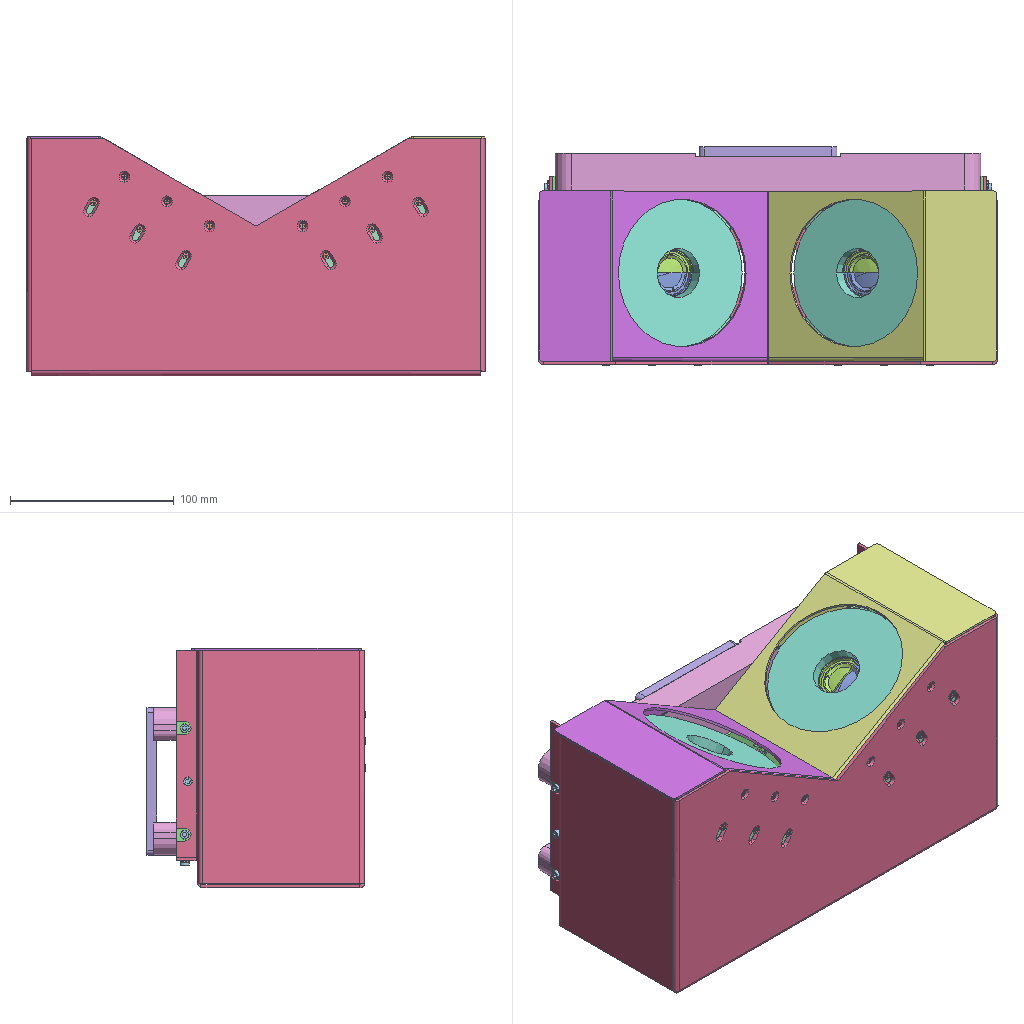Assembly | SolidWorks | 8 different items | 19 placed | box 280 x 133 x 146 mm
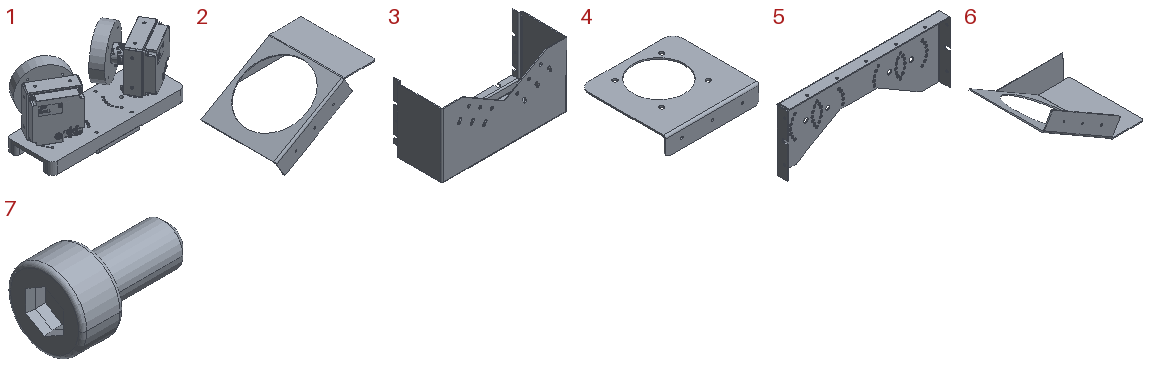Parts list (item | name | quantity | size | volume | features):
1 | (subassembly) | x1 | - | 1121716 mm3 | -
2 | - | x1 | 139.665 x 104 x 75.919 mm | 19261 mm3 | features Cut 2, EdgeFlange 2, Fillet 1, FlatPattern 1, HoleWzd 1, ICE 1, SMBaseFlange 1, SheetMetal 1
3 | - | x1 | 280 x 115 x 145 mm | 201442 mm3 | features Cut 7, EdgeFlange 7, Fillet 2, MirrorPattern 2, Chamfer 1, FlatPattern 1, HoleWzd 1, ICE 1, SMBaseFlange 1, SheetMetal 1, SketchPattern 1
4 | - | x2 | 100 x 92 x 20 mm | 12687 mm3 | features Fillet 2, HoleWzd 2, Cut 1, EdgeFlange 1, FlatPattern 1, ICE 1, SMBaseFlange 1, SheetMetal 1
5 | - | x1 | 263 x 19 x 99.5 mm | 41053 mm3 | features HoleWzd 6, Fillet 4, Cut 3, EdgeFlange 2, MirrorPattern 2, FlatPattern 1, ICE 1, SMBaseFlange 1, SheetMetal 1
6 | - | x1 | 139.665 x 104 x 75.919 mm | 19261 mm3 | features MirrorStock 1
7 | - | x11 | 9 x 5.5 x 5.5 mm | 104.699 mm3 | features Chamfer 2, Fillet 1, ICE 1, Revolution 1
8 | cross recessed ctsk wood screws gb | x1 | - | - | -
Mates (type | each side: item.copy, entity, surface, feature):
Coincident | 1.1 plane | assembly plane | 3 times
Width | 3.1 face plane Edge-Flange1 | 3.1 face plane Edge-Flange1 | 5.1 face plane Edge-Flange1 | 5.1 face plane Edge-Flange1
Concentric | 5.1 face cylinder M3 Clearance Hole2 | 7.1 face cylinder Revolve1
Coincident | 5.1 face plane Edge-Flange1 | 7.1 face plane Revolve1
Concentric | 5.1 face cylinder M3 Clearance Hole2 | 7.2 face cylinder Revolve1
Coincident | 5.1 face plane Edge-Flange1 | 7.2 face plane Revolve1
Concentric | 5.1 face cylinder M3 Clearance Hole1 | 7.3 face cylinder Revolve1
Coincident | 5.1 face plane Edge-Flange1 | 7.3 face plane Revolve1
Concentric | 5.1 face cylinder M3 Clearance Hole1 | 7.4 face cylinder Revolve1
Coincident | 5.1 face plane Edge-Flange1 | 7.4 face plane Revolve1
Concentric | 5.1 face cylinder M3 Clearance Hole1 | 7.5 face cylinder Revolve1
Coincident | 5.1 face plane Edge-Flange1 | 7.5 face plane Revolve1
Concentric | 5.1 face cylinder M3 Clearance Hole2 | 7.6 face cylinder Revolve1
Coincident | 5.1 face plane Edge-Flange1 | 7.6 face plane Revolve1
Concentric | 5.1 face cylinder M3 Clearance Hole2 | 7.7 face cylinder Revolve1
Coincident | 5.1 face plane Edge-Flange1 | 7.7 face plane Revolve1
Concentric | 3.1 face cylinder Cut-Extrude5 | 7.8 face cylinder Revolve1
Coincident | 3.1 face plane Edge-Flange3 | 7.8 face plane Revolve1
Concentric | 3.1 face cylinder Cut-Extrude7 | 7.9 face cylinder Revolve1
Coincident | 3.1 face plane Edge-Flange7 | 7.9 face plane Revolve1
Concentric | 3.1 face cylinder Cut-Extrude7 | 7.10 face cylinder Revolve1
Coincident | 3.1 face plane Edge-Flange7 | 7.10 face plane Revolve1
Concentric | 3.1 face cylinder Cut-Extrude5 | 7.11 face cylinder Revolve1
Coincident | 3.1 face plane Edge-Flange3 | 7.11 face plane Revolve1
Parallel | 5.1 face plane Edge-Flange1 | 3.1 face plane Edge-Flange1
Coincident | 5.1 face plane Edge-Flange1 | 3.1 face plane Edge-Flange7 | 2 times
Parallel | 3.1 face plane Base-Flange1 | 2.1 face plane Base-Flange1
Coincident | 3.1 face plane Base-Flange1 | 2.1 face plane Edge-Flange2
Coincident | 3.1 face plane Cut-Extrude2 | 2.1 face plane Edge-Flange1
Coincident | 3.1 face plane Base-Flange1 | 4.1 face plane Edge-Flange1